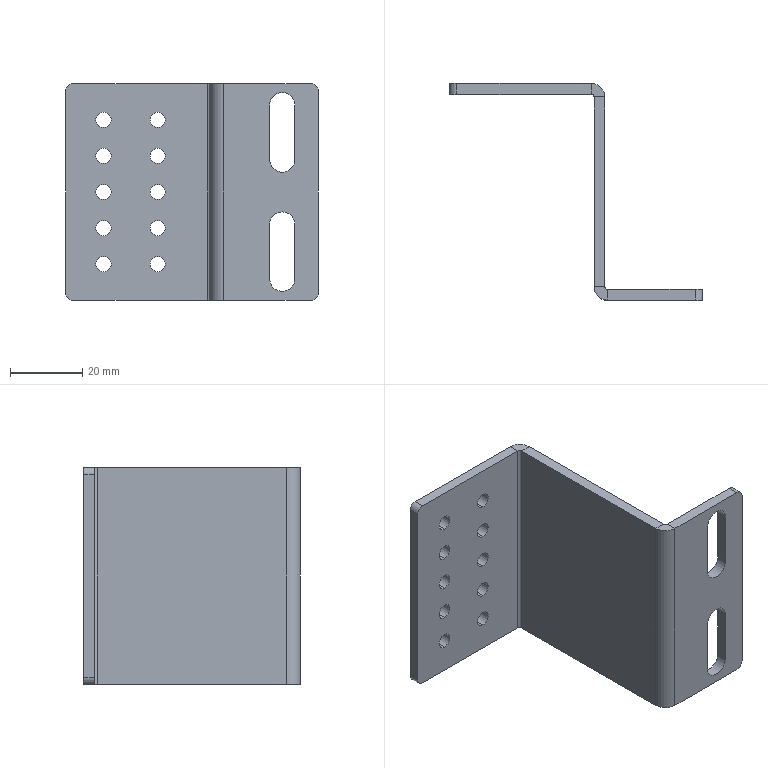Part | STEP file | 11-FG-B09011 | 1 solid | 56 faces | box 70 x 60 x 60 mm | volume 21228 mm3 | cylinder 34 | plane 22 | commonest cylinder face diameters 4.2 x20 7 x6 4 x4 1.473 x2 7.473 x2